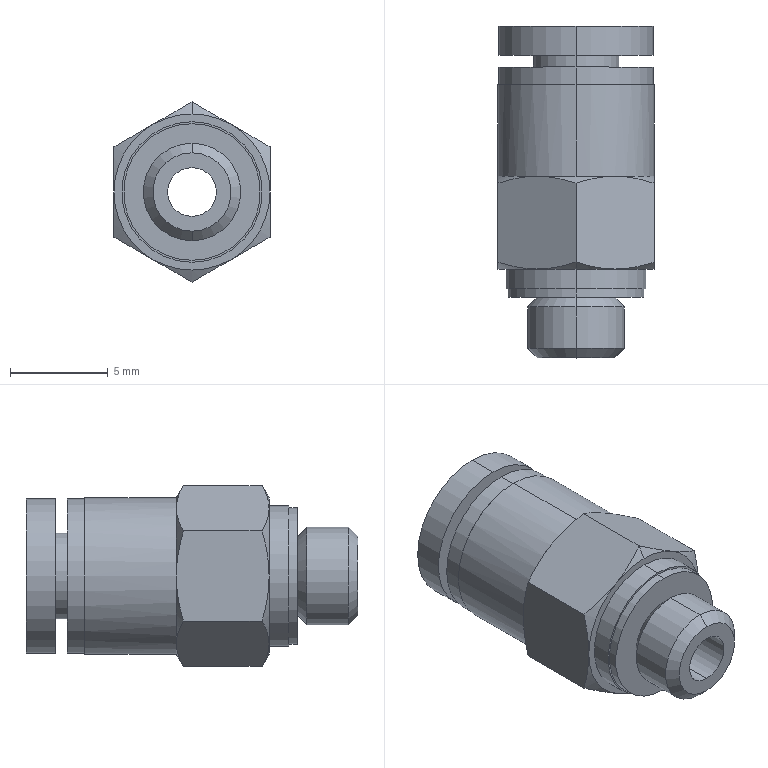Part | STEP file | Quick-change joint KQ2H04-M5A | 1 solid | 51 faces | box 8 x 17 x 9.238 mm | volume 543.469 mm3 | cylinder 18 | cone 18 | plane 15 | commonest cylinder face diameters 7.9 x4 2.5 x2 4.2 x2 4.4 x2 5 x2 7 x2